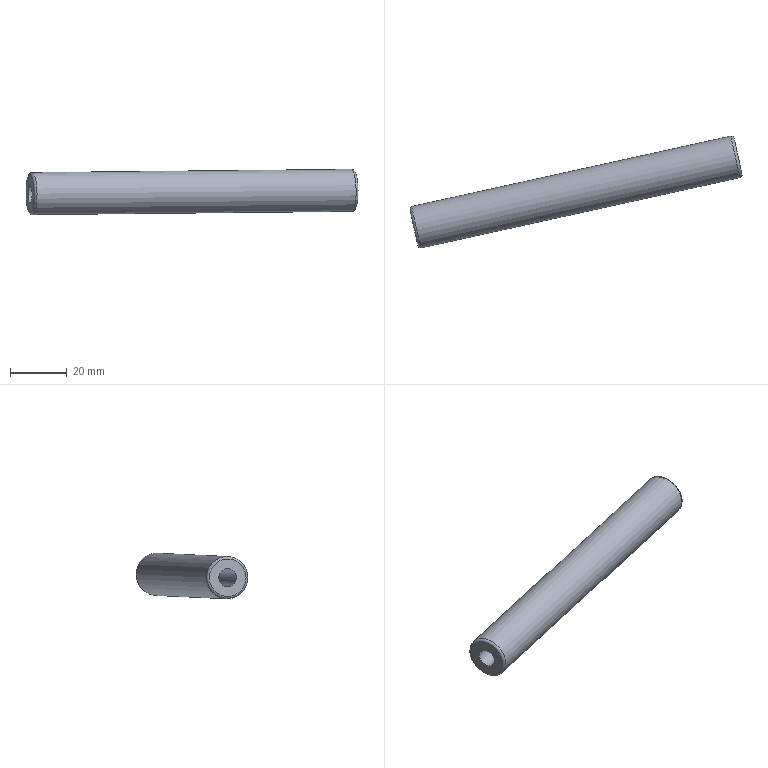Part | NX | features 9416K301(body) 2 | 1 solid | 7 faces | box 117.444 x 39.555 x 16.14 mm | volume 17283 mm3 | plane 3 | cylinder 2 | torus 2 | commonest cylinder face diameters 6.396 x1 14.986 x1
STEP:
#1=CARTESIAN_POINT('',(424.755,-29.066,-86.535));
#2=VERTEX_POINT('',#1);
#3=CARTESIAN_POINT('',(426.183,-35.544,-86.535));
#4=DIRECTION('',(-0.9765,-0.2153,-0.009994));
#5=DIRECTION('',(-0.2153,0.9766,0.));
#6=AXIS2_PLACEMENT_3D('',#3,#4,#5);
#7=CIRCLE('',#6,6.634);
#8=EDGE_CURVE('',#2,#2,#7,.F.);
#9=ORIENTED_EDGE('',*,*,#8,.T.);
#10=EDGE_LOOP('',(#9));
#11=FACE_BOUND('',#10,.T.);
#12=CARTESIAN_POINT('',(426.183,-35.544,-86.535));
#13=DIRECTION('',(-0.9765,-0.2153,-0.009994));
#14=DIRECTION('',(-0.2153,0.9766,0.));
#15=AXIS2_PLACEMENT_3D('',#12,#13,#14);
#16=PLANE('',#15);
#17=ADVANCED_FACE('',(#11),#16,.F.);
#18=CARTESIAN_POINT('',(310.865,-53.292,-87.698));
#19=VERTEX_POINT('',#18);
#20=CARTESIAN_POINT('',(312.478,-60.609,-87.698));
#21=DIRECTION('',(0.9765,0.2153,0.009994));
#22=DIRECTION('',(-0.2153,0.9766,0.));
#23=AXIS2_PLACEMENT_3D('',#20,#21,#22);
#24=CIRCLE('',#23,7.493);
#25=EDGE_CURVE('',#19,#19,#24,.T.);
#26=ORIENTED_EDGE('',*,*,#25,.T.);
#27=EDGE_LOOP('',(#26));
#28=FACE_BOUND('',#27,.T.);
#29=CARTESIAN_POINT('',(423.732,-28.412,-86.543));
#30=VERTEX_POINT('',#29);
#31=CARTESIAN_POINT('',(425.345,-35.729,-86.543));
#32=DIRECTION('',(-0.9765,-0.2153,-0.009994));
#33=DIRECTION('',(-0.2153,0.9766,0.));
#34=AXIS2_PLACEMENT_3D('',#31,#32,#33);
#35=CIRCLE('',#34,7.493);
#36=EDGE_CURVE('',#30,#30,#35,.T.);
#37=ORIENTED_EDGE('',*,*,#36,.T.);
#38=EDGE_LOOP('',(#37));
#39=FACE_BOUND('',#38,.T.);
#40=CARTESIAN_POINT('',(272.155,-69.498,-88.111));
#41=DIRECTION('',(-0.9765,-0.2153,-0.009994));
#42=DIRECTION('',(-0.2153,0.9766,0.));
#43=AXIS2_PLACEMENT_3D('',#40,#41,#42);
#44=CYLINDRICAL_SURFACE('',#43,7.493);
#45=ADVANCED_FACE('',(#28,#39),#44,.T.);
#46=CARTESIAN_POINT('',(310.211,-54.315,-87.707));
#47=VERTEX_POINT('',#46);
#48=CARTESIAN_POINT('',(311.639,-60.794,-87.707));
#49=DIRECTION('',(0.9765,0.2153,0.009994));
#50=DIRECTION('',(-0.2153,0.9766,0.));
#51=AXIS2_PLACEMENT_3D('',#48,#49,#50);
#52=CIRCLE('',#51,6.634);
#53=EDGE_CURVE('',#47,#47,#52,.F.);
#54=ORIENTED_EDGE('',*,*,#53,.T.);
#55=EDGE_LOOP('',(#54));
#56=FACE_BOUND('',#55,.T.);
#57=CARTESIAN_POINT('',(310.951,-57.671,-87.707));
#58=VERTEX_POINT('',#57);
#59=CARTESIAN_POINT('',(311.639,-60.794,-87.707));
#60=DIRECTION('',(0.9765,0.2153,0.009994));
#61=DIRECTION('',(-0.2153,0.9766,0.));
#62=AXIS2_PLACEMENT_3D('',#59,#60,#61);
#63=CIRCLE('',#62,3.198);
#64=EDGE_CURVE('',#58,#58,#63,.F.);
#65=ORIENTED_EDGE('',*,*,#64,.F.);
#66=EDGE_LOOP('',(#65));
#67=FACE_BOUND('',#66,.T.);
#68=CARTESIAN_POINT('',(311.67,-60.787,-90.905));
#69=DIRECTION('',(0.9765,0.2153,0.009994));
#70=DIRECTION('',(0.2153,-0.9766,0.));
#71=AXIS2_PLACEMENT_3D('',#68,#69,#70);
#72=PLANE('',#71);
#73=ADVANCED_FACE('',(#56,#67),#72,.F.);
#74=CARTESIAN_POINT('',(414.066,-34.941,-86.652));
#75=VERTEX_POINT('',#74);
#76=CARTESIAN_POINT('',(414.754,-38.064,-86.652));
#77=DIRECTION('',(0.9765,0.2153,0.009994));
#78=DIRECTION('',(-0.2153,0.9766,0.));
#79=AXIS2_PLACEMENT_3D('',#76,#77,#78);
#80=CIRCLE('',#79,3.198);
#81=EDGE_CURVE('',#75,#75,#80,.F.);
#82=ORIENTED_EDGE('',*,*,#81,.F.);
#83=EDGE_LOOP('',(#82));
#84=FACE_BOUND('',#83,.T.);
#85=ORIENTED_EDGE('',*,*,#64,.T.);
#86=EDGE_LOOP('',(#85));
#87=FACE_BOUND('',#86,.T.);
#88=CARTESIAN_POINT('',(272.155,-69.498,-88.111));
#89=DIRECTION('',(-0.9765,-0.2153,-0.009994));
#90=DIRECTION('',(-0.2153,0.9766,0.));
#91=AXIS2_PLACEMENT_3D('',#88,#89,#90);
#92=CYLINDRICAL_SURFACE('',#91,3.198);
#93=ADVANCED_FACE('',(#84,#87),#92,.F.);
#94=ORIENTED_EDGE('',*,*,#81,.T.);
#95=EDGE_LOOP('',(#94));
#96=FACE_BOUND('',#95,.T.);
#97=CARTESIAN_POINT('',(414.785,-38.057,-89.85));
#98=DIRECTION('',(0.9765,0.2153,0.009994));
#99=DIRECTION('',(0.2153,-0.9766,0.));
#100=AXIS2_PLACEMENT_3D('',#97,#98,#99);
#101=PLANE('',#100);
#102=ADVANCED_FACE('',(#96),#101,.F.);
#103=ORIENTED_EDGE('',*,*,#8,.F.);
#104=EDGE_LOOP('',(#103));
#105=FACE_BOUND('',#104,.T.);
#106=ORIENTED_EDGE('',*,*,#36,.F.);
#107=EDGE_LOOP('',(#106));
#108=FACE_BOUND('',#107,.T.);
#109=CARTESIAN_POINT('',(425.345,-35.729,-86.543));
#110=DIRECTION('',(-0.9765,-0.2153,-0.009994));
#111=DIRECTION('',(-0.2153,0.9766,0.));
#112=AXIS2_PLACEMENT_3D('',#109,#110,#111);
#113=TOROIDAL_SURFACE('',#112,6.634,0.859);
#114=ADVANCED_FACE('',(#105,#108),#113,.T.);
#115=ORIENTED_EDGE('',*,*,#25,.F.);
#116=EDGE_LOOP('',(#115));
#117=FACE_BOUND('',#116,.T.);
#118=ORIENTED_EDGE('',*,*,#53,.F.);
#119=EDGE_LOOP('',(#118));
#120=FACE_BOUND('',#119,.T.);
#121=CARTESIAN_POINT('',(312.478,-60.609,-87.698));
#122=DIRECTION('',(0.9765,0.2153,0.009994));
#123=DIRECTION('',(-0.2153,0.9766,0.));
#124=AXIS2_PLACEMENT_3D('',#121,#122,#123);
#125=TOROIDAL_SURFACE('',#124,6.634,0.859);
#126=ADVANCED_FACE('',(#117,#120),#125,.T.);
#127=CLOSED_SHELL('',(#17,#45,#73,#93,#102,#114,#126));
#128=MANIFOLD_SOLID_BREP('',#127);
#129=(LENGTH_UNIT()NAMED_UNIT(*)SI_UNIT(.MILLI.,.METRE.));
#130=UNCERTAINTY_MEASURE_WITH_UNIT(LENGTH_MEASURE(0.00001),#129,'','');
#131=(NAMED_UNIT(*)PLANE_ANGLE_UNIT()SI_UNIT($,.RADIAN.));
#132=(NAMED_UNIT(*)SI_UNIT($,.STERADIAN.)SOLID_ANGLE_UNIT());
#133=(GEOMETRIC_REPRESENTATION_CONTEXT(3)GLOBAL_UNCERTAINTY_ASSIGNED_CONTEXT((#130))GLOBAL_UNIT_ASSIGNED_CONTEXT((#129,#131,#132))REPRESENTATION_CONTEXT('',''));
#134=ADVANCED_BREP_SHAPE_REPRESENTATION('',(#128),#133);